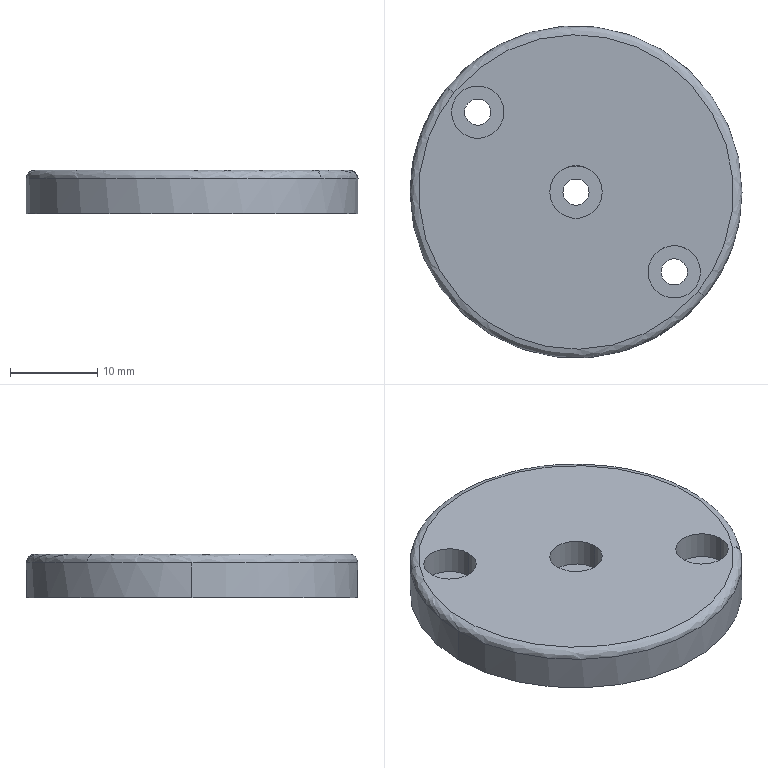Part | SolidWorks | features BaseBody 1 | 1 solid | 21 faces | box 38 x 38 x 5 mm | volume 5337 mm3 | cylinder 14 | plane 5 | spline 2 | commonest cylinder face diameters 3 x6 6 x6 38 x2
STEP:
#1=CARTESIAN_POINT('',(479.235,-109.572,320.545));
#2=VERTEX_POINT('',#1);
#3=CARTESIAN_POINT('',(451.305,-86.858,320.545));
#4=VERTEX_POINT('',#3);
#5=CARTESIAN_POINT('',(479.235,-109.572,320.545));
#6=CARTESIAN_POINT('',(456.522,-137.502,320.545));
#7=CARTESIAN_POINT('',(428.592,-114.788,320.545));
#8=CARTESIAN_POINT('',(451.305,-86.858,320.545));
#9=(BOUNDED_CURVE()B_SPLINE_CURVE(3,(#5,#6,#7,#8),.UNSPECIFIED.,.F.,.T.)B_SPLINE_CURVE_WITH_KNOTS((4,4),(0.,1.),.UNSPECIFIED.)CURVE()GEOMETRIC_REPRESENTATION_ITEM()RATIONAL_B_SPLINE_CURVE((1.,0.3333,0.3333,1.))REPRESENTATION_ITEM(''));
#10=EDGE_CURVE('',#2,#4,#9,.T.);
#11=ORIENTED_EDGE('',*,*,#10,.T.);
#12=CARTESIAN_POINT('',(450.529,-86.227,319.545));
#13=VERTEX_POINT('',#12);
#14=CARTESIAN_POINT('',(451.305,-86.858,319.545));
#15=DIRECTION('',(-0.6309,-0.7758,0.000000012));
#16=DIRECTION('',(-0.7758,0.6309,0.000000021));
#17=AXIS2_PLACEMENT_3D('',#14,#15,#16);
#18=CIRCLE('',#17,1.);
#19=EDGE_CURVE('',#4,#13,#18,.T.);
#20=ORIENTED_EDGE('',*,*,#19,.T.);
#21=CARTESIAN_POINT('',(446.27,-98.215,319.545));
#22=VERTEX_POINT('',#21);
#23=CARTESIAN_POINT('',(465.27,-98.215,319.545));
#24=DIRECTION('',(-0.000000024,0.000000004,-1.));
#25=DIRECTION('',(1.,0.,-0.000000024));
#26=AXIS2_PLACEMENT_3D('',#23,#24,#25);
#27=CIRCLE('',#26,19.);
#28=EDGE_CURVE('',#22,#13,#27,.T.);
#29=ORIENTED_EDGE('',*,*,#28,.F.);
#30=CARTESIAN_POINT('',(480.011,-110.203,319.545));
#31=VERTEX_POINT('',#30);
#32=CARTESIAN_POINT('',(465.27,-98.215,319.545));
#33=DIRECTION('',(-0.000000024,0.000000004,-1.));
#34=DIRECTION('',(1.,0.,-0.000000024));
#35=AXIS2_PLACEMENT_3D('',#32,#33,#34);
#36=CIRCLE('',#35,19.);
#37=EDGE_CURVE('',#31,#22,#36,.T.);
#38=ORIENTED_EDGE('',*,*,#37,.F.);
#39=CARTESIAN_POINT('',(479.235,-109.572,319.545));
#40=DIRECTION('',(0.6309,0.7758,-0.000000012));
#41=DIRECTION('',(0.7758,-0.6309,-0.000000021));
#42=AXIS2_PLACEMENT_3D('',#39,#40,#41);
#43=CIRCLE('',#42,1.);
#44=EDGE_CURVE('',#2,#31,#43,.T.);
#45=ORIENTED_EDGE('',*,*,#44,.F.);
#46=EDGE_LOOP('',(#11,#20,#29,#38,#45));
#47=FACE_OUTER_BOUND('',#46,.T.);
#48=CARTESIAN_POINT('',(451.305,-86.858,320.545));
#49=CARTESIAN_POINT('',(428.592,-114.788,320.545));
#50=CARTESIAN_POINT('',(456.522,-137.502,320.545));
#51=CARTESIAN_POINT('',(479.235,-109.572,320.545));
#52=CARTESIAN_POINT('',(450.851,-86.489,320.545));
#53=CARTESIAN_POINT('',(427.398,-115.328,320.545));
#54=CARTESIAN_POINT('',(456.237,-138.78,320.545));
#55=CARTESIAN_POINT('',(479.69,-109.941,320.545));
#56=CARTESIAN_POINT('',(450.529,-86.227,320.13));
#57=CARTESIAN_POINT('',(426.554,-115.709,320.13));
#58=CARTESIAN_POINT('',(456.036,-139.685,320.13));
#59=CARTESIAN_POINT('',(480.011,-110.203,320.13));
#60=CARTESIAN_POINT('',(450.529,-86.227,319.545));
#61=CARTESIAN_POINT('',(426.554,-115.709,319.545));
#62=CARTESIAN_POINT('',(456.036,-139.685,319.545));
#63=CARTESIAN_POINT('',(480.011,-110.203,319.545));
#64=(BOUNDED_SURFACE()B_SPLINE_SURFACE(3,3,((#48,#49,#50,#51),(#52,#53,#54,#55),(#56,#57,#58,#59),(#60,#61,#62,#63)),.UNSPECIFIED.,.F.,.F.,.F.)B_SPLINE_SURFACE_WITH_KNOTS((4,4),(4,4),(0.,1.),(0.,1.),.UNSPECIFIED.)GEOMETRIC_REPRESENTATION_ITEM()RATIONAL_B_SPLINE_SURFACE(((1.,0.3333,0.3333,1.),(0.8047,0.2682,0.2682,0.8047),(0.8047,0.2682,0.2682,0.8047),(1.,0.3333,0.3333,1.)))REPRESENTATION_ITEM('')SURFACE());
#65=ADVANCED_FACE('',(#47),#64,.T.);
#66=CARTESIAN_POINT('',(446.27,-98.215,315.545));
#67=VERTEX_POINT('',#66);
#68=CARTESIAN_POINT('',(484.27,-98.215,315.545));
#69=VERTEX_POINT('',#68);
#70=CARTESIAN_POINT('',(465.27,-98.215,315.545));
#71=DIRECTION('',(-0.000000024,0.000000004,-1.));
#72=DIRECTION('',(1.,0.,-0.000000024));
#73=AXIS2_PLACEMENT_3D('',#70,#71,#72);
#74=CIRCLE('',#73,19.);
#75=EDGE_CURVE('',#67,#69,#74,.T.);
#76=ORIENTED_EDGE('',*,*,#75,.F.);
#77=CARTESIAN_POINT('',(446.27,-98.215,320.545));
#78=DIRECTION('',(0.000000024,-0.000000004,1.));
#79=VECTOR('',#78,1000.);
#80=LINE('',#77,#79);
#81=EDGE_CURVE('',#67,#22,#80,.T.);
#82=ORIENTED_EDGE('',*,*,#81,.T.);
#83=ORIENTED_EDGE('',*,*,#28,.T.);
#84=CARTESIAN_POINT('',(484.27,-98.215,319.545));
#85=VERTEX_POINT('',#84);
#86=CARTESIAN_POINT('',(465.27,-98.215,319.545));
#87=DIRECTION('',(-0.000000024,0.000000004,-1.));
#88=DIRECTION('',(1.,0.,-0.000000024));
#89=AXIS2_PLACEMENT_3D('',#86,#87,#88);
#90=CIRCLE('',#89,19.);
#91=EDGE_CURVE('',#13,#85,#90,.T.);
#92=ORIENTED_EDGE('',*,*,#91,.T.);
#93=CARTESIAN_POINT('',(484.27,-98.215,320.545));
#94=DIRECTION('',(0.000000024,-0.000000004,1.));
#95=VECTOR('',#94,1000.);
#96=LINE('',#93,#95);
#97=EDGE_CURVE('',#69,#85,#96,.T.);
#98=ORIENTED_EDGE('',*,*,#97,.F.);
#99=EDGE_LOOP('',(#76,#82,#83,#92,#98));
#100=FACE_OUTER_BOUND('',#99,.T.);
#101=CARTESIAN_POINT('',(465.27,-98.215,320.545));
#102=DIRECTION('',(0.000000024,-0.000000004,1.));
#103=DIRECTION('',(1.,0.,-0.000000024));
#104=AXIS2_PLACEMENT_3D('',#101,#102,#103);
#105=CYLINDRICAL_SURFACE('',#104,19.);
#106=ADVANCED_FACE('',(#100),#105,.T.);
#107=CARTESIAN_POINT('',(475.02,-107.363,315.545));
#108=VERTEX_POINT('',#107);
#109=CARTESIAN_POINT('',(478.02,-107.363,315.545));
#110=VERTEX_POINT('',#109);
#111=CARTESIAN_POINT('',(476.52,-107.363,315.545));
#112=DIRECTION('',(0.000000024,-0.000000004,1.));
#113=DIRECTION('',(1.,0.,-0.000000024));
#114=AXIS2_PLACEMENT_3D('',#111,#112,#113);
#115=CIRCLE('',#114,1.5);
#116=EDGE_CURVE('',#108,#110,#115,.T.);
#117=ORIENTED_EDGE('',*,*,#116,.F.);
#118=CARTESIAN_POINT('',(475.02,-107.363,317.37));
#119=VERTEX_POINT('',#118);
#120=CARTESIAN_POINT('',(475.02,-107.363,316.457));
#121=DIRECTION('',(0.000000024,-0.000000004,1.));
#122=VECTOR('',#121,1000.);
#123=LINE('',#120,#122);
#124=EDGE_CURVE('',#108,#119,#123,.T.);
#125=ORIENTED_EDGE('',*,*,#124,.T.);
#126=CARTESIAN_POINT('',(478.02,-107.363,317.37));
#127=VERTEX_POINT('',#126);
#128=CARTESIAN_POINT('',(476.52,-107.363,317.37));
#129=DIRECTION('',(-0.000000024,0.000000004,-1.));
#130=DIRECTION('',(1.,0.,-0.000000024));
#131=AXIS2_PLACEMENT_3D('',#128,#129,#130);
#132=CIRCLE('',#131,1.5);
#133=EDGE_CURVE('',#127,#119,#132,.T.);
#134=ORIENTED_EDGE('',*,*,#133,.F.);
#135=CARTESIAN_POINT('',(478.02,-107.363,316.457));
#136=DIRECTION('',(0.000000024,-0.000000004,1.));
#137=VECTOR('',#136,1000.);
#138=LINE('',#135,#137);
#139=EDGE_CURVE('',#110,#127,#138,.T.);
#140=ORIENTED_EDGE('',*,*,#139,.F.);
#141=EDGE_LOOP('',(#117,#125,#134,#140));
#142=FACE_OUTER_BOUND('',#141,.T.);
#143=CARTESIAN_POINT('',(476.52,-107.363,316.457));
#144=DIRECTION('',(0.000000024,-0.000000004,1.));
#145=DIRECTION('',(1.,0.,-0.000000024));
#146=AXIS2_PLACEMENT_3D('',#143,#144,#145);
#147=CYLINDRICAL_SURFACE('',#146,1.5);
#148=ADVANCED_FACE('',(#142),#147,.F.);
#149=CARTESIAN_POINT('',(452.521,-89.066,315.545));
#150=VERTEX_POINT('',#149);
#151=CARTESIAN_POINT('',(455.521,-89.066,315.545));
#152=VERTEX_POINT('',#151);
#153=CARTESIAN_POINT('',(454.021,-89.066,315.545));
#154=DIRECTION('',(0.000000024,-0.000000004,1.));
#155=DIRECTION('',(1.,0.,-0.000000024));
#156=AXIS2_PLACEMENT_3D('',#153,#154,#155);
#157=CIRCLE('',#156,1.5);
#158=EDGE_CURVE('',#150,#152,#157,.T.);
#159=ORIENTED_EDGE('',*,*,#158,.F.);
#160=CARTESIAN_POINT('',(452.521,-89.066,317.37));
#161=VERTEX_POINT('',#160);
#162=CARTESIAN_POINT('',(452.521,-89.066,316.457));
#163=DIRECTION('',(0.000000024,-0.000000004,1.));
#164=VECTOR('',#163,1000.);
#165=LINE('',#162,#164);
#166=EDGE_CURVE('',#150,#161,#165,.T.);
#167=ORIENTED_EDGE('',*,*,#166,.T.);
#168=CARTESIAN_POINT('',(455.521,-89.066,317.37));
#169=VERTEX_POINT('',#168);
#170=CARTESIAN_POINT('',(454.021,-89.066,317.37));
#171=DIRECTION('',(-0.000000024,0.000000004,-1.));
#172=DIRECTION('',(1.,0.,-0.000000024));
#173=AXIS2_PLACEMENT_3D('',#170,#171,#172);
#174=CIRCLE('',#173,1.5);
#175=EDGE_CURVE('',#169,#161,#174,.T.);
#176=ORIENTED_EDGE('',*,*,#175,.F.);
#177=CARTESIAN_POINT('',(455.521,-89.066,316.457));
#178=DIRECTION('',(0.000000024,-0.000000004,1.));
#179=VECTOR('',#178,1000.);
#180=LINE('',#177,#179);
#181=EDGE_CURVE('',#152,#169,#180,.T.);
#182=ORIENTED_EDGE('',*,*,#181,.F.);
#183=EDGE_LOOP('',(#159,#167,#176,#182));
#184=FACE_OUTER_BOUND('',#183,.T.);
#185=CARTESIAN_POINT('',(454.021,-89.066,316.457));
#186=DIRECTION('',(0.000000024,-0.000000004,1.));
#187=DIRECTION('',(1.,0.,-0.000000024));
#188=AXIS2_PLACEMENT_3D('',#185,#186,#187);
#189=CYLINDRICAL_SURFACE('',#188,1.5);
#190=ADVANCED_FACE('',(#184),#189,.F.);
#191=CARTESIAN_POINT('',(463.77,-98.215,315.545));
#192=VERTEX_POINT('',#191);
#193=CARTESIAN_POINT('',(466.77,-98.215,315.545));
#194=VERTEX_POINT('',#193);
#195=CARTESIAN_POINT('',(465.27,-98.215,315.545));
#196=DIRECTION('',(0.000000024,-0.000000004,1.));
#197=DIRECTION('',(1.,0.,-0.000000024));
#198=AXIS2_PLACEMENT_3D('',#195,#196,#197);
#199=CIRCLE('',#198,1.5);
#200=EDGE_CURVE('',#192,#194,#199,.T.);
#201=ORIENTED_EDGE('',*,*,#200,.F.);
#202=CARTESIAN_POINT('',(463.77,-98.215,317.37));
#203=VERTEX_POINT('',#202);
#204=CARTESIAN_POINT('',(463.77,-98.215,316.457));
#205=DIRECTION('',(0.000000024,-0.000000004,1.));
#206=VECTOR('',#205,1000.);
#207=LINE('',#204,#206);
#208=EDGE_CURVE('',#192,#203,#207,.T.);
#209=ORIENTED_EDGE('',*,*,#208,.T.);
#210=CARTESIAN_POINT('',(466.77,-98.215,317.37));
#211=VERTEX_POINT('',#210);
#212=CARTESIAN_POINT('',(465.27,-98.215,317.37));
#213=DIRECTION('',(-0.000000024,0.000000004,-1.));
#214=DIRECTION('',(1.,0.,-0.000000024));
#215=AXIS2_PLACEMENT_3D('',#212,#213,#214);
#216=CIRCLE('',#215,1.5);
#217=EDGE_CURVE('',#211,#203,#216,.T.);
#218=ORIENTED_EDGE('',*,*,#217,.F.);
#219=CARTESIAN_POINT('',(466.77,-98.215,316.457));
#220=DIRECTION('',(0.000000024,-0.000000004,1.));
#221=VECTOR('',#220,1000.);
#222=LINE('',#219,#221);
#223=EDGE_CURVE('',#194,#211,#222,.T.);
#224=ORIENTED_EDGE('',*,*,#223,.F.);
#225=EDGE_LOOP('',(#201,#209,#218,#224));
#226=FACE_OUTER_BOUND('',#225,.T.);
#227=CARTESIAN_POINT('',(465.27,-98.215,316.457));
#228=DIRECTION('',(0.000000024,-0.000000004,1.));
#229=DIRECTION('',(1.,0.,-0.000000024));
#230=AXIS2_PLACEMENT_3D('',#227,#228,#229);
#231=CYLINDRICAL_SURFACE('',#230,1.5);
#232=ADVANCED_FACE('',(#226),#231,.F.);
#233=CARTESIAN_POINT('',(479.52,-107.363,317.37));
#234=VERTEX_POINT('',#233);
#235=CARTESIAN_POINT('',(473.52,-107.363,317.37));
#236=VERTEX_POINT('',#235);
#237=CARTESIAN_POINT('',(476.52,-107.363,317.37));
#238=DIRECTION('',(-0.000000024,0.000000004,-1.));
#239=DIRECTION('',(1.,0.,-0.000000024));
#240=AXIS2_PLACEMENT_3D('',#237,#238,#239);
#241=CIRCLE('',#240,3.);
#242=EDGE_CURVE('',#234,#236,#241,.T.);
#243=ORIENTED_EDGE('',*,*,#242,.T.);
#244=CARTESIAN_POINT('',(473.52,-107.363,320.545));
#245=VERTEX_POINT('',#244);
#246=CARTESIAN_POINT('',(473.52,-107.363,318.957));
#247=DIRECTION('',(0.000000024,-0.000000004,1.));
#248=VECTOR('',#247,1000.);
#249=LINE('',#246,#248);
#250=EDGE_CURVE('',#236,#245,#249,.T.);
#251=ORIENTED_EDGE('',*,*,#250,.T.);
#252=CARTESIAN_POINT('',(479.52,-107.363,320.545));
#253=VERTEX_POINT('',#252);
#254=CARTESIAN_POINT('',(476.52,-107.363,320.545));
#255=DIRECTION('',(0.000000024,-0.000000004,1.));
#256=DIRECTION('',(1.,0.,-0.000000024));
#257=AXIS2_PLACEMENT_3D('',#254,#255,#256);
#258=CIRCLE('',#257,3.);
#259=EDGE_CURVE('',#245,#253,#258,.T.);
#260=ORIENTED_EDGE('',*,*,#259,.T.);
#261=CARTESIAN_POINT('',(479.52,-107.363,318.957));
#262=DIRECTION('',(0.000000024,-0.000000004,1.));
#263=VECTOR('',#262,1000.);
#264=LINE('',#261,#263);
#265=EDGE_CURVE('',#234,#253,#264,.T.);
#266=ORIENTED_EDGE('',*,*,#265,.F.);
#267=EDGE_LOOP('',(#243,#251,#260,#266));
#268=FACE_OUTER_BOUND('',#267,.T.);
#269=CARTESIAN_POINT('',(476.52,-107.363,318.957));
#270=DIRECTION('',(0.000000024,-0.000000004,1.));
#271=DIRECTION('',(1.,0.,-0.000000024));
#272=AXIS2_PLACEMENT_3D('',#269,#270,#271);
#273=CYLINDRICAL_SURFACE('',#272,3.);
#274=ADVANCED_FACE('',(#268),#273,.F.);
#275=CARTESIAN_POINT('',(457.021,-89.066,317.37));
#276=VERTEX_POINT('',#275);
#277=CARTESIAN_POINT('',(451.021,-89.066,317.37));
#278=VERTEX_POINT('',#277);
#279=CARTESIAN_POINT('',(454.021,-89.066,317.37));
#280=DIRECTION('',(-0.000000024,0.000000004,-1.));
#281=DIRECTION('',(1.,0.,-0.000000024));
#282=AXIS2_PLACEMENT_3D('',#279,#280,#281);
#283=CIRCLE('',#282,3.);
#284=EDGE_CURVE('',#276,#278,#283,.T.);
#285=ORIENTED_EDGE('',*,*,#284,.T.);
#286=CARTESIAN_POINT('',(451.021,-89.066,320.545));
#287=VERTEX_POINT('',#286);
#288=CARTESIAN_POINT('',(451.021,-89.066,318.957));
#289=DIRECTION('',(0.000000024,-0.000000004,1.));
#290=VECTOR('',#289,1000.);
#291=LINE('',#288,#290);
#292=EDGE_CURVE('',#278,#287,#291,.T.);
#293=ORIENTED_EDGE('',*,*,#292,.T.);
#294=CARTESIAN_POINT('',(457.021,-89.066,320.545));
#295=VERTEX_POINT('',#294);
#296=CARTESIAN_POINT('',(454.021,-89.066,320.545));
#297=DIRECTION('',(0.000000024,-0.000000004,1.));
#298=DIRECTION('',(1.,0.,-0.000000024));
#299=AXIS2_PLACEMENT_3D('',#296,#297,#298);
#300=CIRCLE('',#299,3.);
#301=EDGE_CURVE('',#287,#295,#300,.T.);
#302=ORIENTED_EDGE('',*,*,#301,.T.);
#303=CARTESIAN_POINT('',(457.021,-89.066,318.957));
#304=DIRECTION('',(0.000000024,-0.000000004,1.));
#305=VECTOR('',#304,1000.);
#306=LINE('',#303,#305);
#307=EDGE_CURVE('',#276,#295,#306,.T.);
#308=ORIENTED_EDGE('',*,*,#307,.F.);
#309=EDGE_LOOP('',(#285,#293,#302,#308));
#310=FACE_OUTER_BOUND('',#309,.T.);
#311=CARTESIAN_POINT('',(454.021,-89.066,318.957));
#312=DIRECTION('',(0.000000024,-0.000000004,1.));
#313=DIRECTION('',(1.,0.,-0.000000024));
#314=AXIS2_PLACEMENT_3D('',#311,#312,#313);
#315=CYLINDRICAL_SURFACE('',#314,3.);
#316=ADVANCED_FACE('',(#310),#315,.F.);
#317=CARTESIAN_POINT('',(468.27,-98.215,317.37));
#318=VERTEX_POINT('',#317);
#319=CARTESIAN_POINT('',(462.27,-98.215,317.37));
#320=VERTEX_POINT('',#319);
#321=CARTESIAN_POINT('',(465.27,-98.215,317.37));
#322=DIRECTION('',(-0.000000024,0.000000004,-1.));
#323=DIRECTION('',(1.,0.,-0.000000024));
#324=AXIS2_PLACEMENT_3D('',#321,#322,#323);
#325=CIRCLE('',#324,3.);
#326=EDGE_CURVE('',#318,#320,#325,.T.);
#327=ORIENTED_EDGE('',*,*,#326,.T.);
#328=CARTESIAN_POINT('',(462.27,-98.215,320.545));
#329=VERTEX_POINT('',#328);
#330=CARTESIAN_POINT('',(462.27,-98.215,318.957));
#331=DIRECTION('',(0.000000024,-0.000000004,1.));
#332=VECTOR('',#331,1000.);
#333=LINE('',#330,#332);
#334=EDGE_CURVE('',#320,#329,#333,.T.);
#335=ORIENTED_EDGE('',*,*,#334,.T.);
#336=CARTESIAN_POINT('',(468.27,-98.215,320.545));
#337=VERTEX_POINT('',#336);
#338=CARTESIAN_POINT('',(465.27,-98.215,320.545));
#339=DIRECTION('',(0.000000024,-0.000000004,1.));
#340=DIRECTION('',(1.,0.,-0.000000024));
#341=AXIS2_PLACEMENT_3D('',#338,#339,#340);
#342=CIRCLE('',#341,3.);
#343=EDGE_CURVE('',#329,#337,#342,.T.);
#344=ORIENTED_EDGE('',*,*,#343,.T.);
#345=CARTESIAN_POINT('',(468.27,-98.215,318.957));
#346=DIRECTION('',(0.000000024,-0.000000004,1.));
#347=VECTOR('',#346,1000.);
#348=LINE('',#345,#347);
#349=EDGE_CURVE('',#318,#337,#348,.T.);
#350=ORIENTED_EDGE('',*,*,#349,.F.);
#351=EDGE_LOOP('',(#327,#335,#344,#350));
#352=FACE_OUTER_BOUND('',#351,.T.);
#353=CARTESIAN_POINT('',(465.27,-98.215,318.957));
#354=DIRECTION('',(0.000000024,-0.000000004,1.));
#355=DIRECTION('',(1.,0.,-0.000000024));
#356=AXIS2_PLACEMENT_3D('',#353,#354,#355);
#357=CYLINDRICAL_SURFACE('',#356,3.);
#358=ADVANCED_FACE('',(#352),#357,.F.);
#359=CARTESIAN_POINT('',(465.27,-98.215,315.545));
#360=DIRECTION('',(-0.000000024,0.000000004,-1.));
#361=DIRECTION('',(1.,0.,-0.000000024));
#362=AXIS2_PLACEMENT_3D('',#359,#360,#361);
#363=CIRCLE('',#362,19.);
#364=EDGE_CURVE('',#69,#67,#363,.T.);
#365=ORIENTED_EDGE('',*,*,#364,.T.);
#366=ORIENTED_EDGE('',*,*,#75,.T.);
#367=EDGE_LOOP('',(#365,#366));
#368=FACE_OUTER_BOUND('',#367,.T.);
#369=CARTESIAN_POINT('',(476.52,-107.363,315.545));
#370=DIRECTION('',(0.000000024,-0.000000004,1.));
#371=DIRECTION('',(1.,0.,-0.000000024));
#372=AXIS2_PLACEMENT_3D('',#369,#370,#371);
#373=CIRCLE('',#372,1.5);
#374=EDGE_CURVE('',#110,#108,#373,.T.);
#375=ORIENTED_EDGE('',*,*,#374,.T.);
#376=ORIENTED_EDGE('',*,*,#116,.T.);
#377=EDGE_LOOP('',(#375,#376));
#378=FACE_BOUND('',#377,.T.);
#379=CARTESIAN_POINT('',(454.021,-89.066,315.545));
#380=DIRECTION('',(0.000000024,-0.000000004,1.));
#381=DIRECTION('',(1.,0.,-0.000000024));
#382=AXIS2_PLACEMENT_3D('',#379,#380,#381);
#383=CIRCLE('',#382,1.5);
#384=EDGE_CURVE('',#152,#150,#383,.T.);
#385=ORIENTED_EDGE('',*,*,#384,.T.);
#386=ORIENTED_EDGE('',*,*,#158,.T.);
#387=EDGE_LOOP('',(#385,#386));
#388=FACE_BOUND('',#387,.T.);
#389=CARTESIAN_POINT('',(465.27,-98.215,315.545));
#390=DIRECTION('',(0.000000024,-0.000000004,1.));
#391=DIRECTION('',(1.,0.,-0.000000024));
#392=AXIS2_PLACEMENT_3D('',#389,#390,#391);
#393=CIRCLE('',#392,1.5);
#394=EDGE_CURVE('',#194,#192,#393,.T.);
#395=ORIENTED_EDGE('',*,*,#394,.T.);
#396=ORIENTED_EDGE('',*,*,#200,.T.);
#397=EDGE_LOOP('',(#395,#396));
#398=FACE_BOUND('',#397,.T.);
#399=CARTESIAN_POINT('',(465.27,-98.215,315.545));
#400=DIRECTION('',(-0.000000024,0.000000004,-1.));
#401=DIRECTION('',(-1.,0.,0.000000024));
#402=AXIS2_PLACEMENT_3D('',#399,#400,#401);
#403=PLANE('',#402);
#404=ADVANCED_FACE('',(#368,#378,#388,#398),#403,.T.);
#405=ORIENTED_EDGE('',*,*,#81,.F.);
#406=ORIENTED_EDGE('',*,*,#364,.F.);
#407=ORIENTED_EDGE('',*,*,#97,.T.);
#408=CARTESIAN_POINT('',(465.27,-98.215,319.545));
#409=DIRECTION('',(-0.000000024,0.000000004,-1.));
#410=DIRECTION('',(1.,0.,-0.000000024));
#411=AXIS2_PLACEMENT_3D('',#408,#409,#410);
#412=CIRCLE('',#411,19.);
#413=EDGE_CURVE('',#85,#31,#412,.T.);
#414=ORIENTED_EDGE('',*,*,#413,.T.);
#415=ORIENTED_EDGE('',*,*,#37,.T.);
#416=EDGE_LOOP('',(#405,#406,#407,#414,#415));
#417=FACE_OUTER_BOUND('',#416,.T.);
#418=CARTESIAN_POINT('',(465.27,-98.215,320.545));
#419=DIRECTION('',(0.000000024,-0.000000004,1.));
#420=DIRECTION('',(1.,0.,-0.000000024));
#421=AXIS2_PLACEMENT_3D('',#418,#419,#420);
#422=CYLINDRICAL_SURFACE('',#421,19.);
#423=ADVANCED_FACE('',(#417),#422,.T.);
#424=ORIENTED_EDGE('',*,*,#124,.F.);
#425=ORIENTED_EDGE('',*,*,#374,.F.);
#426=ORIENTED_EDGE('',*,*,#139,.T.);
#427=CARTESIAN_POINT('',(476.52,-107.363,317.37));
#428=DIRECTION('',(-0.000000024,0.000000004,-1.));
#429=DIRECTION('',(1.,0.,-0.000000024));
#430=AXIS2_PLACEMENT_3D('',#427,#428,#429);
#431=CIRCLE('',#430,1.5);
#432=EDGE_CURVE('',#119,#127,#431,.T.);
#433=ORIENTED_EDGE('',*,*,#432,.F.);
#434=EDGE_LOOP('',(#424,#425,#426,#433));
#435=FACE_OUTER_BOUND('',#434,.T.);
#436=CARTESIAN_POINT('',(476.52,-107.363,316.457));
#437=DIRECTION('',(0.000000024,-0.000000004,1.));
#438=DIRECTION('',(1.,0.,-0.000000024));
#439=AXIS2_PLACEMENT_3D('',#436,#437,#438);
#440=CYLINDRICAL_SURFACE('',#439,1.5);
#441=ADVANCED_FACE('',(#435),#440,.F.);
#442=ORIENTED_EDGE('',*,*,#166,.F.);
#443=ORIENTED_EDGE('',*,*,#384,.F.);
#444=ORIENTED_EDGE('',*,*,#181,.T.);
#445=CARTESIAN_POINT('',(454.021,-89.066,317.37));
#446=DIRECTION('',(-0.000000024,0.000000004,-1.));
#447=DIRECTION('',(1.,0.,-0.000000024));
#448=AXIS2_PLACEMENT_3D('',#445,#446,#447);
#449=CIRCLE('',#448,1.5);
#450=EDGE_CURVE('',#161,#169,#449,.T.);
#451=ORIENTED_EDGE('',*,*,#450,.F.);
#452=EDGE_LOOP('',(#442,#443,#444,#451));
#453=FACE_OUTER_BOUND('',#452,.T.);
#454=CARTESIAN_POINT('',(454.021,-89.066,316.457));
#455=DIRECTION('',(0.000000024,-0.000000004,1.));
#456=DIRECTION('',(1.,0.,-0.000000024));
#457=AXIS2_PLACEMENT_3D('',#454,#455,#456);
#458=CYLINDRICAL_SURFACE('',#457,1.5);
#459=ADVANCED_FACE('',(#453),#458,.F.);
#460=ORIENTED_EDGE('',*,*,#208,.F.);
#461=ORIENTED_EDGE('',*,*,#394,.F.);
#462=ORIENTED_EDGE('',*,*,#223,.T.);
#463=CARTESIAN_POINT('',(465.27,-98.215,317.37));
#464=DIRECTION('',(-0.000000024,0.000000004,-1.));
#465=DIRECTION('',(1.,0.,-0.000000024));
#466=AXIS2_PLACEMENT_3D('',#463,#464,#465);
#467=CIRCLE('',#466,1.5);
#468=EDGE_CURVE('',#203,#211,#467,.T.);
#469=ORIENTED_EDGE('',*,*,#468,.F.);
#470=EDGE_LOOP('',(#460,#461,#462,#469));
#471=FACE_OUTER_BOUND('',#470,.T.);
#472=CARTESIAN_POINT('',(465.27,-98.215,316.457));
#473=DIRECTION('',(0.000000024,-0.000000004,1.));
#474=DIRECTION('',(1.,0.,-0.000000024));
#475=AXIS2_PLACEMENT_3D('',#472,#473,#474);
#476=CYLINDRICAL_SURFACE('',#475,1.5);
#477=ADVANCED_FACE('',(#471),#476,.F.);
#478=ORIENTED_EDGE('',*,*,#19,.F.);
#479=CARTESIAN_POINT('',(451.305,-86.858,320.545));
#480=CARTESIAN_POINT('',(474.019,-58.928,320.545));
#481=CARTESIAN_POINT('',(501.949,-81.641,320.545));
#482=CARTESIAN_POINT('',(479.235,-109.572,320.545));
#483=(BOUNDED_CURVE()B_SPLINE_CURVE(3,(#479,#480,#481,#482),.UNSPECIFIED.,.F.,.F.)B_SPLINE_CURVE_WITH_KNOTS((4,4),(0.,1.),.UNSPECIFIED.)CURVE()GEOMETRIC_REPRESENTATION_ITEM()RATIONAL_B_SPLINE_CURVE((1.,0.3333,0.3333,1.))REPRESENTATION_ITEM(''));
#484=EDGE_CURVE('',#4,#2,#483,.T.);
#485=ORIENTED_EDGE('',*,*,#484,.T.);
#486=ORIENTED_EDGE('',*,*,#44,.T.);
#487=ORIENTED_EDGE('',*,*,#413,.F.);
#488=ORIENTED_EDGE('',*,*,#91,.F.);
#489=EDGE_LOOP('',(#478,#485,#486,#487,#488));
#490=FACE_OUTER_BOUND('',#489,.T.);
#491=CARTESIAN_POINT('',(479.235,-109.572,320.545));
#492=CARTESIAN_POINT('',(501.949,-81.641,320.545));
#493=CARTESIAN_POINT('',(474.019,-58.928,320.545));
#494=CARTESIAN_POINT('',(451.305,-86.858,320.545));
#495=CARTESIAN_POINT('',(479.69,-109.941,320.545));
#496=CARTESIAN_POINT('',(503.142,-81.102,320.545));
#497=CARTESIAN_POINT('',(474.303,-57.649,320.545));
#498=CARTESIAN_POINT('',(450.851,-86.489,320.545));
#499=CARTESIAN_POINT('',(480.011,-110.203,320.13));
#500=CARTESIAN_POINT('',(503.987,-80.721,320.13));
#501=CARTESIAN_POINT('',(474.505,-56.745,320.13));
#502=CARTESIAN_POINT('',(450.529,-86.227,320.13));
#503=CARTESIAN_POINT('',(480.011,-110.203,319.545));
#504=CARTESIAN_POINT('',(503.987,-80.721,319.545));
#505=CARTESIAN_POINT('',(474.505,-56.745,319.545));
#506=CARTESIAN_POINT('',(450.529,-86.227,319.545));
#507=(BOUNDED_SURFACE()B_SPLINE_SURFACE(3,3,((#491,#492,#493,#494),(#495,#496,#497,#498),(#499,#500,#501,#502),(#503,#504,#505,#506)),.UNSPECIFIED.,.F.,.F.,.F.)B_SPLINE_SURFACE_WITH_KNOTS((4,4),(4,4),(0.,1.),(0.,1.),.UNSPECIFIED.)GEOMETRIC_REPRESENTATION_ITEM()RATIONAL_B_SPLINE_SURFACE(((1.,0.3333,0.3333,1.),(0.8047,0.2682,0.2682,0.8047),(0.8047,0.2682,0.2682,0.8047),(1.,0.3333,0.3333,1.)))REPRESENTATION_ITEM('')SURFACE());
#508=ADVANCED_FACE('',(#490),#507,.T.);
#509=ORIENTED_EDGE('',*,*,#242,.F.);
#510=CARTESIAN_POINT('',(476.52,-107.363,317.37));
#511=DIRECTION('',(-0.000000024,0.000000004,-1.));
#512=DIRECTION('',(1.,0.,-0.000000024));
#513=AXIS2_PLACEMENT_3D('',#510,#511,#512);
#514=CIRCLE('',#513,3.);
#515=EDGE_CURVE('',#236,#234,#514,.T.);
#516=ORIENTED_EDGE('',*,*,#515,.F.);
#517=EDGE_LOOP('',(#509,#516));
#518=FACE_OUTER_BOUND('',#517,.T.);
#519=ORIENTED_EDGE('',*,*,#133,.T.);
#520=ORIENTED_EDGE('',*,*,#432,.T.);
#521=EDGE_LOOP('',(#519,#520));
#522=FACE_BOUND('',#521,.T.);
#523=CARTESIAN_POINT('',(474.774,-105.944,317.37));
#524=DIRECTION('',(-0.000000024,0.000000004,-1.));
#525=DIRECTION('',(-1.,0.,0.000000024));
#526=AXIS2_PLACEMENT_3D('',#523,#524,#525);
#527=PLANE('',#526);
#528=ADVANCED_FACE('',(#518,#522),#527,.F.);
#529=ORIENTED_EDGE('',*,*,#284,.F.);
#530=CARTESIAN_POINT('',(454.021,-89.066,317.37));
#531=DIRECTION('',(-0.000000024,0.000000004,-1.));
#532=DIRECTION('',(1.,0.,-0.000000024));
#533=AXIS2_PLACEMENT_3D('',#530,#531,#532);
#534=CIRCLE('',#533,3.);
#535=EDGE_CURVE('',#278,#276,#534,.T.);
#536=ORIENTED_EDGE('',*,*,#535,.F.);
#537=EDGE_LOOP('',(#529,#536));
#538=FACE_OUTER_BOUND('',#537,.T.);
#539=ORIENTED_EDGE('',*,*,#175,.T.);
#540=ORIENTED_EDGE('',*,*,#450,.T.);
#541=EDGE_LOOP('',(#539,#540));
#542=FACE_BOUND('',#541,.T.);
#543=CARTESIAN_POINT('',(455.766,-90.486,317.37));
#544=DIRECTION('',(-0.000000024,0.000000004,-1.));
#545=DIRECTION('',(-1.,0.,0.000000024));
#546=AXIS2_PLACEMENT_3D('',#543,#544,#545);
#547=PLANE('',#546);
#548=ADVANCED_FACE('',(#538,#542),#547,.F.);
#549=ORIENTED_EDGE('',*,*,#326,.F.);
#550=CARTESIAN_POINT('',(465.27,-98.215,317.37));
#551=DIRECTION('',(-0.000000024,0.000000004,-1.));
#552=DIRECTION('',(1.,0.,-0.000000024));
#553=AXIS2_PLACEMENT_3D('',#550,#551,#552);
#554=CIRCLE('',#553,3.);
#555=EDGE_CURVE('',#320,#318,#554,.T.);
#556=ORIENTED_EDGE('',*,*,#555,.F.);
#557=EDGE_LOOP('',(#549,#556));
#558=FACE_OUTER_BOUND('',#557,.T.);
#559=ORIENTED_EDGE('',*,*,#217,.T.);
#560=ORIENTED_EDGE('',*,*,#468,.T.);
#561=EDGE_LOOP('',(#559,#560));
#562=FACE_BOUND('',#561,.T.);
#563=CARTESIAN_POINT('',(467.016,-99.635,317.37));
#564=DIRECTION('',(-0.000000024,0.000000004,-1.));
#565=DIRECTION('',(-1.,0.,0.000000024));
#566=AXIS2_PLACEMENT_3D('',#563,#564,#565);
#567=PLANE('',#566);
#568=ADVANCED_FACE('',(#558,#562),#567,.F.);
#569=ORIENTED_EDGE('',*,*,#10,.F.);
#570=ORIENTED_EDGE('',*,*,#484,.F.);
#571=EDGE_LOOP('',(#569,#570));
#572=FACE_OUTER_BOUND('',#571,.T.);
#573=CARTESIAN_POINT('',(476.52,-107.363,320.545));
#574=DIRECTION('',(0.000000024,-0.000000004,1.));
#575=DIRECTION('',(1.,0.,-0.000000024));
#576=AXIS2_PLACEMENT_3D('',#573,#574,#575);
#577=CIRCLE('',#576,3.);
#578=EDGE_CURVE('',#253,#245,#577,.T.);
#579=ORIENTED_EDGE('',*,*,#578,.F.);
#580=ORIENTED_EDGE('',*,*,#259,.F.);
#581=EDGE_LOOP('',(#579,#580));
#582=FACE_BOUND('',#581,.T.);
#583=CARTESIAN_POINT('',(454.021,-89.066,320.545));
#584=DIRECTION('',(0.000000024,-0.000000004,1.));
#585=DIRECTION('',(1.,0.,-0.000000024));
#586=AXIS2_PLACEMENT_3D('',#583,#584,#585);
#587=CIRCLE('',#586,3.);
#588=EDGE_CURVE('',#295,#287,#587,.T.);
#589=ORIENTED_EDGE('',*,*,#588,.F.);
#590=ORIENTED_EDGE('',*,*,#301,.F.);
#591=EDGE_LOOP('',(#589,#590));
#592=FACE_BOUND('',#591,.T.);
#593=CARTESIAN_POINT('',(465.27,-98.215,320.545));
#594=DIRECTION('',(0.000000024,-0.000000004,1.));
#595=DIRECTION('',(1.,0.,-0.000000024));
#596=AXIS2_PLACEMENT_3D('',#593,#594,#595);
#597=CIRCLE('',#596,3.);
#598=EDGE_CURVE('',#337,#329,#597,.T.);
#599=ORIENTED_EDGE('',*,*,#598,.F.);
#600=ORIENTED_EDGE('',*,*,#343,.F.);
#601=EDGE_LOOP('',(#599,#600));
#602=FACE_BOUND('',#601,.T.);
#603=CARTESIAN_POINT('',(465.27,-98.215,320.545));
#604=DIRECTION('',(-0.000000024,0.000000004,-1.));
#605=DIRECTION('',(-1.,0.,0.000000024));
#606=AXIS2_PLACEMENT_3D('',#603,#604,#605);
#607=PLANE('',#606);
#608=ADVANCED_FACE('',(#572,#582,#592,#602),#607,.F.);
#609=ORIENTED_EDGE('',*,*,#250,.F.);
#610=ORIENTED_EDGE('',*,*,#515,.T.);
#611=ORIENTED_EDGE('',*,*,#265,.T.);
#612=ORIENTED_EDGE('',*,*,#578,.T.);
#613=EDGE_LOOP('',(#609,#610,#611,#612));
#614=FACE_OUTER_BOUND('',#613,.T.);
#615=CARTESIAN_POINT('',(476.52,-107.363,318.957));
#616=DIRECTION('',(0.000000024,-0.000000004,1.));
#617=DIRECTION('',(1.,0.,-0.000000024));
#618=AXIS2_PLACEMENT_3D('',#615,#616,#617);
#619=CYLINDRICAL_SURFACE('',#618,3.);
#620=ADVANCED_FACE('',(#614),#619,.F.);
#621=ORIENTED_EDGE('',*,*,#292,.F.);
#622=ORIENTED_EDGE('',*,*,#535,.T.);
#623=ORIENTED_EDGE('',*,*,#307,.T.);
#624=ORIENTED_EDGE('',*,*,#588,.T.);
#625=EDGE_LOOP('',(#621,#622,#623,#624));
#626=FACE_OUTER_BOUND('',#625,.T.);
#627=CARTESIAN_POINT('',(454.021,-89.066,318.957));
#628=DIRECTION('',(0.000000024,-0.000000004,1.));
#629=DIRECTION('',(1.,0.,-0.000000024));
#630=AXIS2_PLACEMENT_3D('',#627,#628,#629);
#631=CYLINDRICAL_SURFACE('',#630,3.);
#632=ADVANCED_FACE('',(#626),#631,.F.);
#633=ORIENTED_EDGE('',*,*,#334,.F.);
#634=ORIENTED_EDGE('',*,*,#555,.T.);
#635=ORIENTED_EDGE('',*,*,#349,.T.);
#636=ORIENTED_EDGE('',*,*,#598,.T.);
#637=EDGE_LOOP('',(#633,#634,#635,#636));
#638=FACE_OUTER_BOUND('',#637,.T.);
#639=CARTESIAN_POINT('',(465.27,-98.215,318.957));
#640=DIRECTION('',(0.000000024,-0.000000004,1.));
#641=DIRECTION('',(1.,0.,-0.000000024));
#642=AXIS2_PLACEMENT_3D('',#639,#640,#641);
#643=CYLINDRICAL_SURFACE('',#642,3.);
#644=ADVANCED_FACE('',(#638),#643,.F.);
#645=CLOSED_SHELL('',(#65,#106,#148,#190,#232,#274,#316,#358,#404,#423,#441,#459,#477,#508,#528,#548,#568,#608,#620,#632,#644));
#646=MANIFOLD_SOLID_BREP('',#645);
#647=CARTESIAN_POINT('',(0.,0.,0.));
#648=DIRECTION('',(0.,0.,1.));
#649=DIRECTION('',(1.,0.,0.));
#650=AXIS2_PLACEMENT_3D('',#647,#648,#649);
#651=(LENGTH_UNIT()NAMED_UNIT(*)SI_UNIT(.MILLI.,.METRE.));
#652=UNCERTAINTY_MEASURE_WITH_UNIT(LENGTH_MEASURE(0.00001),#651,'','');
#653=(NAMED_UNIT(*)PLANE_ANGLE_UNIT()SI_UNIT($,.RADIAN.));
#654=(NAMED_UNIT(*)SI_UNIT($,.STERADIAN.)SOLID_ANGLE_UNIT());
#655=(GEOMETRIC_REPRESENTATION_CONTEXT(3)GLOBAL_UNCERTAINTY_ASSIGNED_CONTEXT((#652))GLOBAL_UNIT_ASSIGNED_CONTEXT((#651,#653,#654))REPRESENTATION_CONTEXT('',''));
#656=ADVANCED_BREP_SHAPE_REPRESENTATION('',(#646,#650),#655);